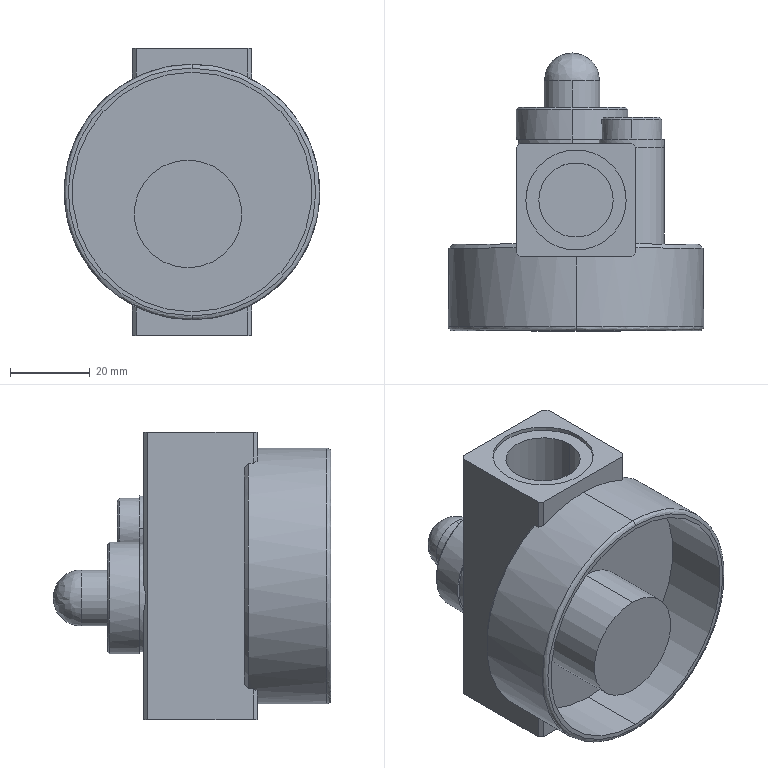Part | STEP file | _BL-4000 Sw | 1 solid | 62 faces | box 64 x 69.32 x 72 mm | volume 89554 mm3 | plane 28 | cylinder 23 | cone 8 | spline 3 | commonest cylinder face diameters 18.631 x4 25.146 x4 27 x4 14 x2 15 x2 28 x2